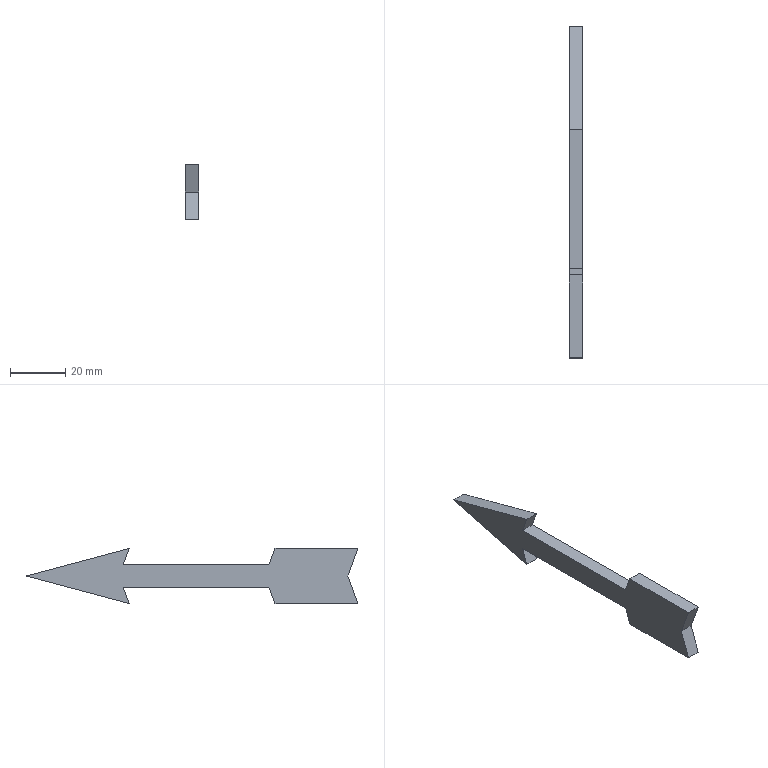Part | NX | features solid 2 | 1 solid | 14 faces | box 5 x 120 x 20 mm | volume 6791 mm3 | plane 14
STEP:
#1=CARTESIAN_POINT('',(2255.,-850.,-650.));
#2=VERTEX_POINT('',#1);
#3=CARTESIAN_POINT('',(2255.,-847.816,-644.));
#4=VERTEX_POINT('',#3);
#5=CARTESIAN_POINT('',(2255.,-848.908,-647.));
#6=DIRECTION('',(0.,0.342,0.9397));
#7=VECTOR('',#6,1000.);
#8=LINE('',#5,#7);
#9=EDGE_CURVE('',#2,#4,#8,.T.);
#10=ORIENTED_EDGE('',*,*,#9,.T.);
#11=CARTESIAN_POINT('',(2255.,-795.137,-644.));
#12=VERTEX_POINT('',#11);
#13=CARTESIAN_POINT('',(2255.,-821.476,-644.));
#14=DIRECTION('',(0.,1.,0.));
#15=VECTOR('',#14,1000.);
#16=LINE('',#13,#15);
#17=EDGE_CURVE('',#4,#12,#16,.T.);
#18=ORIENTED_EDGE('',*,*,#17,.T.);
#19=CARTESIAN_POINT('',(2255.,-797.321,-650.));
#20=VERTEX_POINT('',#19);
#21=CARTESIAN_POINT('',(2255.,-796.229,-647.));
#22=DIRECTION('',(0.,0.342,0.9397));
#23=VECTOR('',#22,1000.);
#24=LINE('',#21,#23);
#25=EDGE_CURVE('',#20,#12,#24,.T.);
#26=ORIENTED_EDGE('',*,*,#25,.F.);
#27=CARTESIAN_POINT('',(2255.,-760.,-640.));
#28=VERTEX_POINT('',#27);
#29=CARTESIAN_POINT('',(2255.,-778.66,-645.));
#30=DIRECTION('',(0.,0.9659,0.2588));
#31=VECTOR('',#30,1000.);
#32=LINE('',#29,#31);
#33=EDGE_CURVE('',#20,#28,#32,.T.);
#34=ORIENTED_EDGE('',*,*,#33,.T.);
#35=CARTESIAN_POINT('',(2255.,-797.321,-630.));
#36=VERTEX_POINT('',#35);
#37=CARTESIAN_POINT('',(2255.,-778.66,-635.));
#38=DIRECTION('',(0.,0.9659,-0.2588));
#39=VECTOR('',#38,1000.);
#40=LINE('',#37,#39);
#41=EDGE_CURVE('',#36,#28,#40,.T.);
#42=ORIENTED_EDGE('',*,*,#41,.F.);
#43=CARTESIAN_POINT('',(2255.,-795.137,-636.));
#44=VERTEX_POINT('',#43);
#45=CARTESIAN_POINT('',(2255.,-796.229,-633.));
#46=DIRECTION('',(0.,0.342,-0.9397));
#47=VECTOR('',#46,1000.);
#48=LINE('',#45,#47);
#49=EDGE_CURVE('',#36,#44,#48,.T.);
#50=ORIENTED_EDGE('',*,*,#49,.T.);
#51=CARTESIAN_POINT('',(2255.,-847.816,-636.));
#52=VERTEX_POINT('',#51);
#53=CARTESIAN_POINT('',(2255.,-821.476,-636.));
#54=DIRECTION('',(0.,1.,0.));
#55=VECTOR('',#54,1000.);
#56=LINE('',#53,#55);
#57=EDGE_CURVE('',#52,#44,#56,.T.);
#58=ORIENTED_EDGE('',*,*,#57,.F.);
#59=CARTESIAN_POINT('',(2255.,-850.,-630.));
#60=VERTEX_POINT('',#59);
#61=CARTESIAN_POINT('',(2255.,-848.908,-633.));
#62=DIRECTION('',(0.,0.342,-0.9397));
#63=VECTOR('',#62,1000.);
#64=LINE('',#61,#63);
#65=EDGE_CURVE('',#60,#52,#64,.T.);
#66=ORIENTED_EDGE('',*,*,#65,.F.);
#67=CARTESIAN_POINT('',(2255.,-880.,-630.));
#68=VERTEX_POINT('',#67);
#69=CARTESIAN_POINT('',(2255.,-865.,-630.));
#70=DIRECTION('',(0.,1.,0.));
#71=VECTOR('',#70,1000.);
#72=LINE('',#69,#71);
#73=EDGE_CURVE('',#68,#60,#72,.T.);
#74=ORIENTED_EDGE('',*,*,#73,.F.);
#75=CARTESIAN_POINT('',(2255.,-876.36,-640.));
#76=VERTEX_POINT('',#75);
#77=CARTESIAN_POINT('',(2255.,-878.18,-635.));
#78=DIRECTION('',(0.,0.342,-0.9397));
#79=VECTOR('',#78,1000.);
#80=LINE('',#77,#79);
#81=EDGE_CURVE('',#68,#76,#80,.T.);
#82=ORIENTED_EDGE('',*,*,#81,.T.);
#83=CARTESIAN_POINT('',(2255.,-880.,-650.));
#84=VERTEX_POINT('',#83);
#85=CARTESIAN_POINT('',(2255.,-878.18,-645.));
#86=DIRECTION('',(0.,0.342,0.9397));
#87=VECTOR('',#86,1000.);
#88=LINE('',#85,#87);
#89=EDGE_CURVE('',#84,#76,#88,.T.);
#90=ORIENTED_EDGE('',*,*,#89,.F.);
#91=CARTESIAN_POINT('',(2255.,-865.,-650.));
#92=DIRECTION('',(0.,1.,0.));
#93=VECTOR('',#92,1000.);
#94=LINE('',#91,#93);
#95=EDGE_CURVE('',#84,#2,#94,.T.);
#96=ORIENTED_EDGE('',*,*,#95,.T.);
#97=EDGE_LOOP('',(#10,#18,#26,#34,#42,#50,#58,#66,#74,#82,#90,#96));
#98=FACE_BOUND('',#97,.T.);
#99=CARTESIAN_POINT('',(2255.,-880.,-590.));
#100=DIRECTION('',(1.,0.,0.));
#101=DIRECTION('',(0.,0.,1.));
#102=AXIS2_PLACEMENT_3D('',#99,#100,#101);
#103=PLANE('',#102);
#104=ADVANCED_FACE('',(#98),#103,.T.);
#105=CARTESIAN_POINT('',(2250.,-880.,-650.));
#106=VERTEX_POINT('',#105);
#107=CARTESIAN_POINT('',(2255.,-880.,-650.));
#108=DIRECTION('',(-1.,0.,0.));
#109=VECTOR('',#108,1000.);
#110=LINE('',#107,#109);
#111=EDGE_CURVE('',#84,#106,#110,.T.);
#112=ORIENTED_EDGE('',*,*,#111,.T.);
#113=CARTESIAN_POINT('',(2250.,-850.,-650.));
#114=VERTEX_POINT('',#113);
#115=CARTESIAN_POINT('',(2250.,-1631.154,-650.));
#116=DIRECTION('',(0.,1.,0.));
#117=VECTOR('',#116,1000.);
#118=LINE('',#115,#117);
#119=EDGE_CURVE('',#106,#114,#118,.T.);
#120=ORIENTED_EDGE('',*,*,#119,.T.);
#121=CARTESIAN_POINT('',(2255.,-850.,-650.));
#122=DIRECTION('',(-1.,0.,0.));
#123=VECTOR('',#122,1000.);
#124=LINE('',#121,#123);
#125=EDGE_CURVE('',#2,#114,#124,.T.);
#126=ORIENTED_EDGE('',*,*,#125,.F.);
#127=ORIENTED_EDGE('',*,*,#95,.F.);
#128=EDGE_LOOP('',(#112,#120,#126,#127));
#129=FACE_BOUND('',#128,.T.);
#130=CARTESIAN_POINT('',(2255.,-865.,-650.));
#131=DIRECTION('',(0.,0.,1.));
#132=DIRECTION('',(0.,-1.,0.));
#133=AXIS2_PLACEMENT_3D('',#130,#131,#132);
#134=PLANE('',#133);
#135=ADVANCED_FACE('',(#129),#134,.F.);
#136=CARTESIAN_POINT('',(2250.,-876.36,-640.));
#137=VERTEX_POINT('',#136);
#138=CARTESIAN_POINT('',(2250.,-878.18,-645.));
#139=DIRECTION('',(0.,-0.342,-0.9397));
#140=VECTOR('',#139,1000.);
#141=LINE('',#138,#140);
#142=EDGE_CURVE('',#137,#106,#141,.T.);
#143=ORIENTED_EDGE('',*,*,#142,.T.);
#144=ORIENTED_EDGE('',*,*,#111,.F.);
#145=ORIENTED_EDGE('',*,*,#89,.T.);
#146=CARTESIAN_POINT('',(2255.,-876.36,-640.));
#147=DIRECTION('',(-1.,0.,0.));
#148=VECTOR('',#147,1000.);
#149=LINE('',#146,#148);
#150=EDGE_CURVE('',#76,#137,#149,.T.);
#151=ORIENTED_EDGE('',*,*,#150,.T.);
#152=EDGE_LOOP('',(#143,#144,#145,#151));
#153=FACE_BOUND('',#152,.T.);
#154=CARTESIAN_POINT('',(2255.,-878.18,-645.));
#155=DIRECTION('',(0.,-0.9397,0.342));
#156=DIRECTION('',(0.,-0.342,-0.9397));
#157=AXIS2_PLACEMENT_3D('',#154,#155,#156);
#158=PLANE('',#157);
#159=ADVANCED_FACE('',(#153),#158,.T.);
#160=CARTESIAN_POINT('',(2250.,-880.,-630.));
#161=VERTEX_POINT('',#160);
#162=CARTESIAN_POINT('',(2255.,-880.,-630.));
#163=DIRECTION('',(-1.,0.,0.));
#164=VECTOR('',#163,1000.);
#165=LINE('',#162,#164);
#166=EDGE_CURVE('',#68,#161,#165,.T.);
#167=ORIENTED_EDGE('',*,*,#166,.T.);
#168=CARTESIAN_POINT('',(2250.,-878.18,-635.));
#169=DIRECTION('',(0.,-0.342,0.9397));
#170=VECTOR('',#169,1000.);
#171=LINE('',#168,#170);
#172=EDGE_CURVE('',#137,#161,#171,.T.);
#173=ORIENTED_EDGE('',*,*,#172,.F.);
#174=ORIENTED_EDGE('',*,*,#150,.F.);
#175=ORIENTED_EDGE('',*,*,#81,.F.);
#176=EDGE_LOOP('',(#167,#173,#174,#175));
#177=FACE_BOUND('',#176,.T.);
#178=CARTESIAN_POINT('',(2255.,-878.18,-635.));
#179=DIRECTION('',(0.,0.9397,0.342));
#180=DIRECTION('',(0.,-0.342,0.9397));
#181=AXIS2_PLACEMENT_3D('',#178,#179,#180);
#182=PLANE('',#181);
#183=ADVANCED_FACE('',(#177),#182,.F.);
#184=CARTESIAN_POINT('',(2250.,-850.,-630.));
#185=VERTEX_POINT('',#184);
#186=CARTESIAN_POINT('',(2250.,-865.,-630.));
#187=DIRECTION('',(0.,-1.,0.));
#188=VECTOR('',#187,1000.);
#189=LINE('',#186,#188);
#190=EDGE_CURVE('',#185,#161,#189,.T.);
#191=ORIENTED_EDGE('',*,*,#190,.T.);
#192=ORIENTED_EDGE('',*,*,#166,.F.);
#193=ORIENTED_EDGE('',*,*,#73,.T.);
#194=CARTESIAN_POINT('',(2255.,-850.,-630.));
#195=DIRECTION('',(-1.,0.,0.));
#196=VECTOR('',#195,1000.);
#197=LINE('',#194,#196);
#198=EDGE_CURVE('',#60,#185,#197,.T.);
#199=ORIENTED_EDGE('',*,*,#198,.T.);
#200=EDGE_LOOP('',(#191,#192,#193,#199));
#201=FACE_BOUND('',#200,.T.);
#202=CARTESIAN_POINT('',(2255.,-865.,-630.));
#203=DIRECTION('',(0.,0.,1.));
#204=DIRECTION('',(0.,-1.,0.));
#205=AXIS2_PLACEMENT_3D('',#202,#203,#204);
#206=PLANE('',#205);
#207=ADVANCED_FACE('',(#201),#206,.T.);
#208=CARTESIAN_POINT('',(2250.,-847.816,-636.));
#209=VERTEX_POINT('',#208);
#210=CARTESIAN_POINT('',(2250.,-848.908,-633.));
#211=DIRECTION('',(0.,-0.342,0.9397));
#212=VECTOR('',#211,1000.);
#213=LINE('',#210,#212);
#214=EDGE_CURVE('',#209,#185,#213,.T.);
#215=ORIENTED_EDGE('',*,*,#214,.T.);
#216=ORIENTED_EDGE('',*,*,#198,.F.);
#217=ORIENTED_EDGE('',*,*,#65,.T.);
#218=CARTESIAN_POINT('',(2255.,-847.816,-636.));
#219=DIRECTION('',(-1.,0.,0.));
#220=VECTOR('',#219,1000.);
#221=LINE('',#218,#220);
#222=EDGE_CURVE('',#52,#209,#221,.T.);
#223=ORIENTED_EDGE('',*,*,#222,.T.);
#224=EDGE_LOOP('',(#215,#216,#217,#223));
#225=FACE_BOUND('',#224,.T.);
#226=CARTESIAN_POINT('',(2255.,-848.908,-633.));
#227=DIRECTION('',(0.,0.9397,0.342));
#228=DIRECTION('',(0.,-0.342,0.9397));
#229=AXIS2_PLACEMENT_3D('',#226,#227,#228);
#230=PLANE('',#229);
#231=ADVANCED_FACE('',(#225),#230,.T.);
#232=CARTESIAN_POINT('',(2250.,-795.137,-636.));
#233=VERTEX_POINT('',#232);
#234=CARTESIAN_POINT('',(2250.,-821.476,-636.));
#235=DIRECTION('',(0.,-1.,0.));
#236=VECTOR('',#235,1000.);
#237=LINE('',#234,#236);
#238=EDGE_CURVE('',#233,#209,#237,.T.);
#239=ORIENTED_EDGE('',*,*,#238,.T.);
#240=ORIENTED_EDGE('',*,*,#222,.F.);
#241=ORIENTED_EDGE('',*,*,#57,.T.);
#242=CARTESIAN_POINT('',(2255.,-795.137,-636.));
#243=DIRECTION('',(-1.,0.,0.));
#244=VECTOR('',#243,1000.);
#245=LINE('',#242,#244);
#246=EDGE_CURVE('',#44,#233,#245,.T.);
#247=ORIENTED_EDGE('',*,*,#246,.T.);
#248=EDGE_LOOP('',(#239,#240,#241,#247));
#249=FACE_BOUND('',#248,.T.);
#250=CARTESIAN_POINT('',(2255.,-821.476,-636.));
#251=DIRECTION('',(0.,0.,1.));
#252=DIRECTION('',(0.,-1.,0.));
#253=AXIS2_PLACEMENT_3D('',#250,#251,#252);
#254=PLANE('',#253);
#255=ADVANCED_FACE('',(#249),#254,.T.);
#256=CARTESIAN_POINT('',(2250.,-797.321,-630.));
#257=VERTEX_POINT('',#256);
#258=CARTESIAN_POINT('',(2255.,-797.321,-630.));
#259=DIRECTION('',(-1.,0.,0.));
#260=VECTOR('',#259,1000.);
#261=LINE('',#258,#260);
#262=EDGE_CURVE('',#36,#257,#261,.T.);
#263=ORIENTED_EDGE('',*,*,#262,.T.);
#264=CARTESIAN_POINT('',(2250.,-796.229,-633.));
#265=DIRECTION('',(0.,-0.342,0.9397));
#266=VECTOR('',#265,1000.);
#267=LINE('',#264,#266);
#268=EDGE_CURVE('',#233,#257,#267,.T.);
#269=ORIENTED_EDGE('',*,*,#268,.F.);
#270=ORIENTED_EDGE('',*,*,#246,.F.);
#271=ORIENTED_EDGE('',*,*,#49,.F.);
#272=EDGE_LOOP('',(#263,#269,#270,#271));
#273=FACE_BOUND('',#272,.T.);
#274=CARTESIAN_POINT('',(2255.,-796.229,-633.));
#275=DIRECTION('',(0.,0.9397,0.342));
#276=DIRECTION('',(0.,-0.342,0.9397));
#277=AXIS2_PLACEMENT_3D('',#274,#275,#276);
#278=PLANE('',#277);
#279=ADVANCED_FACE('',(#273),#278,.F.);
#280=CARTESIAN_POINT('',(2250.,-760.,-640.));
#281=VERTEX_POINT('',#280);
#282=CARTESIAN_POINT('',(2250.,-778.66,-635.));
#283=DIRECTION('',(0.,-0.9659,0.2588));
#284=VECTOR('',#283,1000.);
#285=LINE('',#282,#284);
#286=EDGE_CURVE('',#281,#257,#285,.T.);
#287=ORIENTED_EDGE('',*,*,#286,.T.);
#288=ORIENTED_EDGE('',*,*,#262,.F.);
#289=ORIENTED_EDGE('',*,*,#41,.T.);
#290=CARTESIAN_POINT('',(2255.,-760.,-640.));
#291=DIRECTION('',(-1.,0.,0.));
#292=VECTOR('',#291,1000.);
#293=LINE('',#290,#292);
#294=EDGE_CURVE('',#28,#281,#293,.T.);
#295=ORIENTED_EDGE('',*,*,#294,.T.);
#296=EDGE_LOOP('',(#287,#288,#289,#295));
#297=FACE_BOUND('',#296,.T.);
#298=CARTESIAN_POINT('',(2255.,-778.66,-635.));
#299=DIRECTION('',(0.,0.2588,0.9659));
#300=DIRECTION('',(0.,-0.9659,0.2588));
#301=AXIS2_PLACEMENT_3D('',#298,#299,#300);
#302=PLANE('',#301);
#303=ADVANCED_FACE('',(#297),#302,.T.);
#304=CARTESIAN_POINT('',(2250.,-797.321,-650.));
#305=VERTEX_POINT('',#304);
#306=CARTESIAN_POINT('',(2255.,-797.321,-650.));
#307=DIRECTION('',(-1.,0.,0.));
#308=VECTOR('',#307,1000.);
#309=LINE('',#306,#308);
#310=EDGE_CURVE('',#20,#305,#309,.T.);
#311=ORIENTED_EDGE('',*,*,#310,.T.);
#312=CARTESIAN_POINT('',(2250.,-778.66,-645.));
#313=DIRECTION('',(0.,-0.9659,-0.2588));
#314=VECTOR('',#313,1000.);
#315=LINE('',#312,#314);
#316=EDGE_CURVE('',#281,#305,#315,.T.);
#317=ORIENTED_EDGE('',*,*,#316,.F.);
#318=ORIENTED_EDGE('',*,*,#294,.F.);
#319=ORIENTED_EDGE('',*,*,#33,.F.);
#320=EDGE_LOOP('',(#311,#317,#318,#319));
#321=FACE_BOUND('',#320,.T.);
#322=CARTESIAN_POINT('',(2255.,-778.66,-645.));
#323=DIRECTION('',(0.,-0.2588,0.9659));
#324=DIRECTION('',(0.,-0.9659,-0.2588));
#325=AXIS2_PLACEMENT_3D('',#322,#323,#324);
#326=PLANE('',#325);
#327=ADVANCED_FACE('',(#321),#326,.F.);
#328=CARTESIAN_POINT('',(2250.,-795.137,-644.));
#329=VERTEX_POINT('',#328);
#330=CARTESIAN_POINT('',(2250.,-796.229,-647.));
#331=DIRECTION('',(0.,-0.342,-0.9397));
#332=VECTOR('',#331,1000.);
#333=LINE('',#330,#332);
#334=EDGE_CURVE('',#329,#305,#333,.T.);
#335=ORIENTED_EDGE('',*,*,#334,.T.);
#336=ORIENTED_EDGE('',*,*,#310,.F.);
#337=ORIENTED_EDGE('',*,*,#25,.T.);
#338=CARTESIAN_POINT('',(2255.,-795.137,-644.));
#339=DIRECTION('',(-1.,0.,0.));
#340=VECTOR('',#339,1000.);
#341=LINE('',#338,#340);
#342=EDGE_CURVE('',#12,#329,#341,.T.);
#343=ORIENTED_EDGE('',*,*,#342,.T.);
#344=EDGE_LOOP('',(#335,#336,#337,#343));
#345=FACE_BOUND('',#344,.T.);
#346=CARTESIAN_POINT('',(2255.,-796.229,-647.));
#347=DIRECTION('',(0.,-0.9397,0.342));
#348=DIRECTION('',(0.,-0.342,-0.9397));
#349=AXIS2_PLACEMENT_3D('',#346,#347,#348);
#350=PLANE('',#349);
#351=ADVANCED_FACE('',(#345),#350,.T.);
#352=CARTESIAN_POINT('',(2250.,-847.816,-644.));
#353=VERTEX_POINT('',#352);
#354=CARTESIAN_POINT('',(2255.,-847.816,-644.));
#355=DIRECTION('',(-1.,0.,0.));
#356=VECTOR('',#355,1000.);
#357=LINE('',#354,#356);
#358=EDGE_CURVE('',#4,#353,#357,.T.);
#359=ORIENTED_EDGE('',*,*,#358,.T.);
#360=CARTESIAN_POINT('',(2250.,-821.476,-644.));
#361=DIRECTION('',(0.,-1.,0.));
#362=VECTOR('',#361,1000.);
#363=LINE('',#360,#362);
#364=EDGE_CURVE('',#329,#353,#363,.T.);
#365=ORIENTED_EDGE('',*,*,#364,.F.);
#366=ORIENTED_EDGE('',*,*,#342,.F.);
#367=ORIENTED_EDGE('',*,*,#17,.F.);
#368=EDGE_LOOP('',(#359,#365,#366,#367));
#369=FACE_BOUND('',#368,.T.);
#370=CARTESIAN_POINT('',(2255.,-821.476,-644.));
#371=DIRECTION('',(0.,0.,1.));
#372=DIRECTION('',(0.,-1.,0.));
#373=AXIS2_PLACEMENT_3D('',#370,#371,#372);
#374=PLANE('',#373);
#375=ADVANCED_FACE('',(#369),#374,.F.);
#376=ORIENTED_EDGE('',*,*,#125,.T.);
#377=CARTESIAN_POINT('',(2250.,-848.908,-647.));
#378=DIRECTION('',(0.,-0.342,-0.9397));
#379=VECTOR('',#378,1000.);
#380=LINE('',#377,#379);
#381=EDGE_CURVE('',#353,#114,#380,.T.);
#382=ORIENTED_EDGE('',*,*,#381,.F.);
#383=ORIENTED_EDGE('',*,*,#358,.F.);
#384=ORIENTED_EDGE('',*,*,#9,.F.);
#385=EDGE_LOOP('',(#376,#382,#383,#384));
#386=FACE_BOUND('',#385,.T.);
#387=CARTESIAN_POINT('',(2255.,-848.908,-647.));
#388=DIRECTION('',(0.,-0.9397,0.342));
#389=DIRECTION('',(0.,-0.342,-0.9397));
#390=AXIS2_PLACEMENT_3D('',#387,#388,#389);
#391=PLANE('',#390);
#392=ADVANCED_FACE('',(#386),#391,.F.);
#393=ORIENTED_EDGE('',*,*,#364,.T.);
#394=ORIENTED_EDGE('',*,*,#381,.T.);
#395=ORIENTED_EDGE('',*,*,#119,.F.);
#396=ORIENTED_EDGE('',*,*,#142,.F.);
#397=ORIENTED_EDGE('',*,*,#172,.T.);
#398=ORIENTED_EDGE('',*,*,#190,.F.);
#399=ORIENTED_EDGE('',*,*,#214,.F.);
#400=ORIENTED_EDGE('',*,*,#238,.F.);
#401=ORIENTED_EDGE('',*,*,#268,.T.);
#402=ORIENTED_EDGE('',*,*,#286,.F.);
#403=ORIENTED_EDGE('',*,*,#316,.T.);
#404=ORIENTED_EDGE('',*,*,#334,.F.);
#405=EDGE_LOOP('',(#393,#394,#395,#396,#397,#398,#399,#400,#401,#402,#403,#404));
#406=FACE_BOUND('',#405,.T.);
#407=CARTESIAN_POINT('',(2250.,-876.36,-640.));
#408=DIRECTION('',(-1.,0.,0.));
#409=DIRECTION('',(0.,0.,1.));
#410=AXIS2_PLACEMENT_3D('',#407,#408,#409);
#411=PLANE('',#410);
#412=ADVANCED_FACE('',(#406),#411,.T.);
#413=CLOSED_SHELL('',(#104,#135,#159,#183,#207,#231,#255,#279,#303,#327,#351,#375,#392,#412));
#414=MANIFOLD_SOLID_BREP('',#413);
#415=(LENGTH_UNIT()NAMED_UNIT(*)SI_UNIT(.MILLI.,.METRE.));
#416=UNCERTAINTY_MEASURE_WITH_UNIT(LENGTH_MEASURE(0.00001),#415,'','');
#417=(NAMED_UNIT(*)PLANE_ANGLE_UNIT()SI_UNIT($,.RADIAN.));
#418=(NAMED_UNIT(*)SI_UNIT($,.STERADIAN.)SOLID_ANGLE_UNIT());
#419=(GEOMETRIC_REPRESENTATION_CONTEXT(3)GLOBAL_UNCERTAINTY_ASSIGNED_CONTEXT((#416))GLOBAL_UNIT_ASSIGNED_CONTEXT((#415,#417,#418))REPRESENTATION_CONTEXT('',''));
#420=ADVANCED_BREP_SHAPE_REPRESENTATION('',(#414),#419);